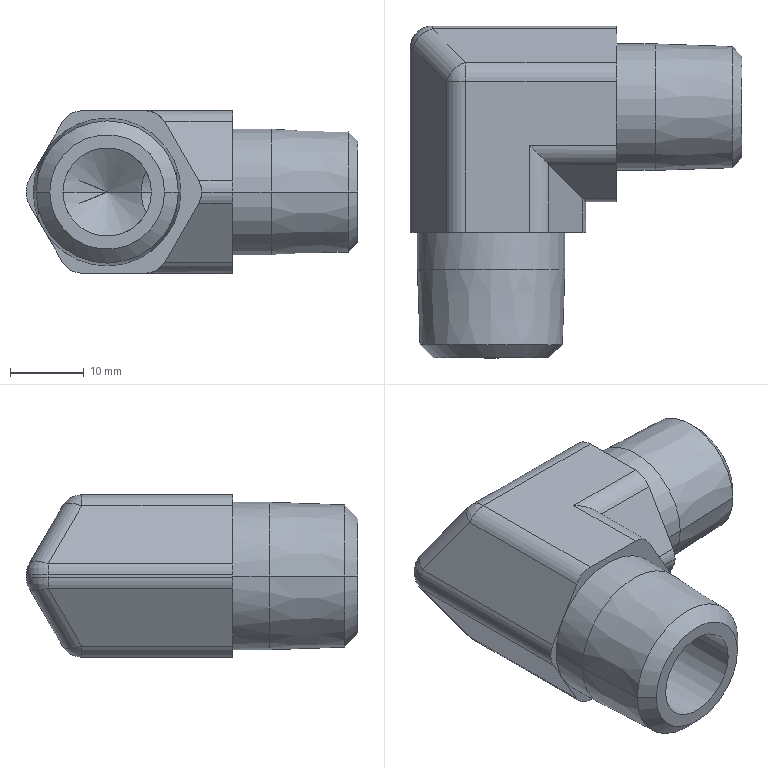Part | STEP file | 4-20.sldasm-Part-133 | 1 solid | 57 faces | box 45 x 45 x 22 mm | volume 14976 mm3 | cylinder 26 | plane 17 | cone 10 | sphere 4 | commonest cylinder face diameters 6 x18 10.3 x2 12 x2 17.145 x2 20 x2